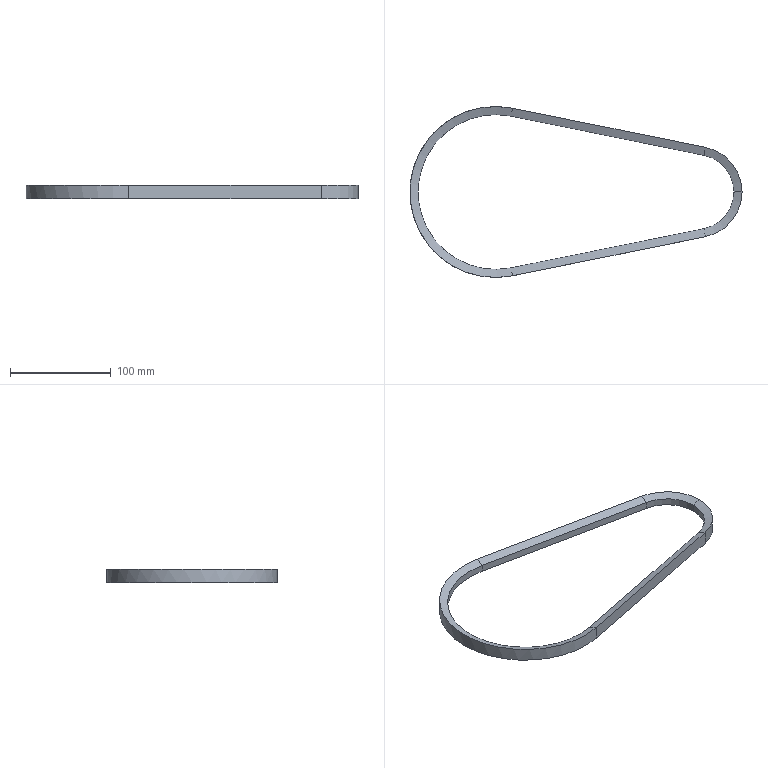Part | SolidWorks | features Sweep 1 | 1 solid | 20 faces | box 329.455 x 169.695 x 13 mm | volume 63968 mm3 | plane 8 | cone 6 | cylinder 6 | commonest cylinder face diameters 74.495 x2 90.495 x2 153.695 x1 169.695 x1
STEP:
#1=CARTESIAN_POINT('',(-184.095,75.316,-3.588));
#2=VERTEX_POINT('',#1);
#3=CARTESIAN_POINT('',(-276.207,0.,-3.588));
#4=VERTEX_POINT('',#3);
#5=CARTESIAN_POINT('',(-199.36,0.,-3.588));
#6=DIRECTION('',(0.,0.,1.));
#7=DIRECTION('',(1.,0.,0.));
#8=AXIS2_PLACEMENT_3D('',#5,#6,#7);
#9=CIRCLE('',#8,76.847);
#10=EDGE_CURVE('',#2,#4,#9,.T.);
#11=ORIENTED_EDGE('',*,*,#10,.T.);
#12=CARTESIAN_POINT('',(-284.207,0.,-6.5));
#13=VERTEX_POINT('',#12);
#14=CARTESIAN_POINT('',(-276.207,0.,-3.588));
#15=DIRECTION('',(-0.9397,0.,-0.342));
#16=VECTOR('',#15,1000.);
#17=LINE('',#14,#16);
#18=EDGE_CURVE('',#4,#13,#17,.T.);
#19=ORIENTED_EDGE('',*,*,#18,.T.);
#20=CARTESIAN_POINT('',(-182.506,83.157,-6.5));
#21=VERTEX_POINT('',#20);
#22=CARTESIAN_POINT('',(-199.36,0.,-6.5));
#23=DIRECTION('',(0.,0.,1.));
#24=DIRECTION('',(1.,0.,0.));
#25=AXIS2_PLACEMENT_3D('',#22,#23,#24);
#26=CIRCLE('',#25,84.847);
#27=EDGE_CURVE('',#21,#13,#26,.T.);
#28=ORIENTED_EDGE('',*,*,#27,.F.);
#29=CARTESIAN_POINT('',(-183.052,80.464,-5.5));
#30=DIRECTION('',(0.1867,0.921,-0.342));
#31=VECTOR('',#30,1000.);
#32=LINE('',#29,#31);
#33=EDGE_CURVE('',#2,#21,#32,.T.);
#34=ORIENTED_EDGE('',*,*,#33,.F.);
#35=EDGE_LOOP('',(#11,#19,#28,#34));
#36=FACE_OUTER_BOUND('',#35,.T.);
#37=CARTESIAN_POINT('',(-199.36,0.,-3.588));
#38=DIRECTION('',(0.,0.,-1.));
#39=DIRECTION('',(-1.,0.,0.));
#40=AXIS2_PLACEMENT_3D('',#37,#38,#39);
#41=CONICAL_SURFACE('',#40,76.847,1.222);
#42=ADVANCED_FACE('',(#36),#41,.F.);
#43=CARTESIAN_POINT('',(8.988,-44.346,-6.5));
#44=VERTEX_POINT('',#43);
#45=CARTESIAN_POINT('',(45.247,0.,-6.5));
#46=VERTEX_POINT('',#45);
#47=CARTESIAN_POINT('',(0.,0.,-6.5));
#48=DIRECTION('',(0.,0.,1.));
#49=DIRECTION('',(1.,0.,0.));
#50=AXIS2_PLACEMENT_3D('',#47,#48,#49);
#51=CIRCLE('',#50,45.247);
#52=EDGE_CURVE('',#44,#46,#51,.T.);
#53=ORIENTED_EDGE('',*,*,#52,.T.);
#54=CARTESIAN_POINT('',(45.247,0.,6.5));
#55=VERTEX_POINT('',#54);
#56=CARTESIAN_POINT('',(45.247,0.,0.));
#57=DIRECTION('',(0.,0.,1.));
#58=VECTOR('',#57,1000.);
#59=LINE('',#56,#58);
#60=EDGE_CURVE('',#46,#55,#59,.T.);
#61=ORIENTED_EDGE('',*,*,#60,.T.);
#62=CARTESIAN_POINT('',(8.988,-44.346,6.5));
#63=VERTEX_POINT('',#62);
#64=CARTESIAN_POINT('',(0.,0.,6.5));
#65=DIRECTION('',(0.,0.,1.));
#66=DIRECTION('',(1.,0.,0.));
#67=AXIS2_PLACEMENT_3D('',#64,#65,#66);
#68=CIRCLE('',#67,45.247);
#69=EDGE_CURVE('',#63,#55,#68,.T.);
#70=ORIENTED_EDGE('',*,*,#69,.F.);
#71=CARTESIAN_POINT('',(8.988,-44.346,-6.5));
#72=DIRECTION('',(0.,0.,1.));
#73=VECTOR('',#72,1000.);
#74=LINE('',#71,#73);
#75=EDGE_CURVE('',#44,#63,#74,.T.);
#76=ORIENTED_EDGE('',*,*,#75,.F.);
#77=EDGE_LOOP('',(#53,#61,#70,#76));
#78=FACE_OUTER_BOUND('',#77,.T.);
#79=CARTESIAN_POINT('',(0.,0.,0.));
#80=DIRECTION('',(0.,0.,1.));
#81=DIRECTION('',(1.,0.,0.));
#82=AXIS2_PLACEMENT_3D('',#79,#80,#81);
#83=CYLINDRICAL_SURFACE('',#82,45.247);
#84=ADVANCED_FACE('',(#78),#83,.T.);
#85=CARTESIAN_POINT('',(37.247,0.,3.588));
#86=VERTEX_POINT('',#85);
#87=CARTESIAN_POINT('',(7.399,36.505,3.588));
#88=VERTEX_POINT('',#87);
#89=CARTESIAN_POINT('',(0.,0.,3.588));
#90=DIRECTION('',(0.,0.,1.));
#91=DIRECTION('',(1.,0.,0.));
#92=AXIS2_PLACEMENT_3D('',#89,#90,#91);
#93=CIRCLE('',#92,37.247);
#94=EDGE_CURVE('',#86,#88,#93,.T.);
#95=ORIENTED_EDGE('',*,*,#94,.F.);
#96=CARTESIAN_POINT('',(45.247,0.,6.5));
#97=DIRECTION('',(0.9397,0.,0.342));
#98=VECTOR('',#97,1000.);
#99=LINE('',#96,#98);
#100=EDGE_CURVE('',#86,#55,#99,.T.);
#101=ORIENTED_EDGE('',*,*,#100,.T.);
#102=CARTESIAN_POINT('',(8.988,44.346,6.5));
#103=VERTEX_POINT('',#102);
#104=CARTESIAN_POINT('',(0.,0.,6.5));
#105=DIRECTION('',(0.,0.,1.));
#106=DIRECTION('',(1.,0.,0.));
#107=AXIS2_PLACEMENT_3D('',#104,#105,#106);
#108=CIRCLE('',#107,45.247);
#109=EDGE_CURVE('',#55,#103,#108,.T.);
#110=ORIENTED_EDGE('',*,*,#109,.T.);
#111=CARTESIAN_POINT('',(8.442,41.653,5.5));
#112=VERTEX_POINT('',#111);
#113=CARTESIAN_POINT('',(8.988,44.346,6.5));
#114=CARTESIAN_POINT('',(8.806,43.448,6.167));
#115=CARTESIAN_POINT('',(8.624,42.551,5.833));
#116=CARTESIAN_POINT('',(8.442,41.653,5.5));
#117=B_SPLINE_CURVE_WITH_KNOTS('',3,(#113,#114,#115,#116),.UNSPECIFIED.,.F.,.F.,(4,4),(0.,1.),.UNSPECIFIED.);
#118=EDGE_CURVE('',#103,#112,#117,.T.);
#119=ORIENTED_EDGE('',*,*,#118,.T.);
#120=CARTESIAN_POINT('',(8.442,41.653,5.5));
#121=CARTESIAN_POINT('',(8.094,39.937,4.863));
#122=CARTESIAN_POINT('',(7.746,38.221,4.225));
#123=CARTESIAN_POINT('',(7.399,36.505,3.588));
#124=B_SPLINE_CURVE_WITH_KNOTS('',3,(#120,#121,#122,#123),.UNSPECIFIED.,.F.,.F.,(4,4),(0.,1.),.UNSPECIFIED.);
#125=EDGE_CURVE('',#112,#88,#124,.T.);
#126=ORIENTED_EDGE('',*,*,#125,.T.);
#127=EDGE_LOOP('',(#95,#101,#110,#119,#126));
#128=FACE_OUTER_BOUND('',#127,.T.);
#129=CARTESIAN_POINT('',(0.,0.,6.5));
#130=DIRECTION('',(0.,0.,1.));
#131=DIRECTION('',(1.,0.,0.));
#132=AXIS2_PLACEMENT_3D('',#129,#130,#131);
#133=CONICAL_SURFACE('',#132,45.247,1.222);
#134=ADVANCED_FACE('',(#128),#133,.F.);
#135=CARTESIAN_POINT('',(37.247,0.,-3.588));
#136=VERTEX_POINT('',#135);
#137=CARTESIAN_POINT('',(7.399,36.505,-3.588));
#138=VERTEX_POINT('',#137);
#139=CARTESIAN_POINT('',(0.,0.,-3.588));
#140=DIRECTION('',(0.,0.,1.));
#141=DIRECTION('',(1.,0.,0.));
#142=AXIS2_PLACEMENT_3D('',#139,#140,#141);
#143=CIRCLE('',#142,37.247);
#144=EDGE_CURVE('',#136,#138,#143,.T.);
#145=ORIENTED_EDGE('',*,*,#144,.F.);
#146=CARTESIAN_POINT('',(37.247,0.,0.));
#147=DIRECTION('',(0.,0.,1.));
#148=VECTOR('',#147,1000.);
#149=LINE('',#146,#148);
#150=EDGE_CURVE('',#136,#86,#149,.T.);
#151=ORIENTED_EDGE('',*,*,#150,.T.);
#152=ORIENTED_EDGE('',*,*,#94,.T.);
#153=CARTESIAN_POINT('',(7.399,36.505,3.588));
#154=CARTESIAN_POINT('',(7.399,36.505,1.196));
#155=CARTESIAN_POINT('',(7.399,36.505,-1.196));
#156=CARTESIAN_POINT('',(7.399,36.505,-3.588));
#157=B_SPLINE_CURVE_WITH_KNOTS('',3,(#153,#154,#155,#156),.UNSPECIFIED.,.F.,.F.,(4,4),(0.,1.),.UNSPECIFIED.);
#158=EDGE_CURVE('',#88,#138,#157,.T.);
#159=ORIENTED_EDGE('',*,*,#158,.T.);
#160=EDGE_LOOP('',(#145,#151,#152,#159));
#161=FACE_OUTER_BOUND('',#160,.T.);
#162=CARTESIAN_POINT('',(0.,0.,0.));
#163=DIRECTION('',(0.,0.,1.));
#164=DIRECTION('',(1.,0.,0.));
#165=AXIS2_PLACEMENT_3D('',#162,#163,#164);
#166=CYLINDRICAL_SURFACE('',#165,37.247);
#167=ADVANCED_FACE('',(#161),#166,.F.);
#168=ORIENTED_EDGE('',*,*,#150,.F.);
#169=CARTESIAN_POINT('',(7.399,-36.505,-3.588));
#170=VERTEX_POINT('',#169);
#171=CARTESIAN_POINT('',(0.,0.,-3.588));
#172=DIRECTION('',(0.,0.,1.));
#173=DIRECTION('',(1.,0.,0.));
#174=AXIS2_PLACEMENT_3D('',#171,#172,#173);
#175=CIRCLE('',#174,37.247);
#176=EDGE_CURVE('',#170,#136,#175,.T.);
#177=ORIENTED_EDGE('',*,*,#176,.F.);
#178=CARTESIAN_POINT('',(7.399,-36.505,3.588));
#179=VERTEX_POINT('',#178);
#180=CARTESIAN_POINT('',(7.399,-36.505,3.588));
#181=DIRECTION('',(0.,0.,-1.));
#182=VECTOR('',#181,1000.);
#183=LINE('',#180,#182);
#184=EDGE_CURVE('',#179,#170,#183,.T.);
#185=ORIENTED_EDGE('',*,*,#184,.F.);
#186=CARTESIAN_POINT('',(0.,0.,3.588));
#187=DIRECTION('',(0.,0.,1.));
#188=DIRECTION('',(1.,0.,0.));
#189=AXIS2_PLACEMENT_3D('',#186,#187,#188);
#190=CIRCLE('',#189,37.247);
#191=EDGE_CURVE('',#179,#86,#190,.T.);
#192=ORIENTED_EDGE('',*,*,#191,.T.);
#193=EDGE_LOOP('',(#168,#177,#185,#192));
#194=FACE_OUTER_BOUND('',#193,.T.);
#195=CARTESIAN_POINT('',(0.,0.,0.));
#196=DIRECTION('',(0.,0.,1.));
#197=DIRECTION('',(1.,0.,0.));
#198=AXIS2_PLACEMENT_3D('',#195,#196,#197);
#199=CYLINDRICAL_SURFACE('',#198,37.247);
#200=ADVANCED_FACE('',(#194),#199,.F.);
#201=ORIENTED_EDGE('',*,*,#100,.F.);
#202=ORIENTED_EDGE('',*,*,#191,.F.);
#203=CARTESIAN_POINT('',(8.442,-41.653,5.5));
#204=DIRECTION('',(-0.1867,0.921,-0.342));
#205=VECTOR('',#204,1000.);
#206=LINE('',#203,#205);
#207=EDGE_CURVE('',#63,#179,#206,.T.);
#208=ORIENTED_EDGE('',*,*,#207,.F.);
#209=ORIENTED_EDGE('',*,*,#69,.T.);
#210=EDGE_LOOP('',(#201,#202,#208,#209));
#211=FACE_OUTER_BOUND('',#210,.T.);
#212=CARTESIAN_POINT('',(0.,0.,6.5));
#213=DIRECTION('',(0.,0.,1.));
#214=DIRECTION('',(1.,0.,0.));
#215=AXIS2_PLACEMENT_3D('',#212,#213,#214);
#216=CONICAL_SURFACE('',#215,45.247,1.222);
#217=ADVANCED_FACE('',(#211),#216,.F.);
#218=ORIENTED_EDGE('',*,*,#60,.F.);
#219=CARTESIAN_POINT('',(8.988,44.346,-6.5));
#220=VERTEX_POINT('',#219);
#221=CARTESIAN_POINT('',(0.,0.,-6.5));
#222=DIRECTION('',(0.,0.,1.));
#223=DIRECTION('',(1.,0.,0.));
#224=AXIS2_PLACEMENT_3D('',#221,#222,#223);
#225=CIRCLE('',#224,45.247);
#226=EDGE_CURVE('',#46,#220,#225,.T.);
#227=ORIENTED_EDGE('',*,*,#226,.T.);
#228=CARTESIAN_POINT('',(8.988,44.346,-6.5));
#229=CARTESIAN_POINT('',(8.988,44.346,-2.167));
#230=CARTESIAN_POINT('',(8.988,44.346,2.167));
#231=CARTESIAN_POINT('',(8.988,44.346,6.5));
#232=B_SPLINE_CURVE_WITH_KNOTS('',3,(#228,#229,#230,#231),.UNSPECIFIED.,.F.,.F.,(4,4),(0.,1.),.UNSPECIFIED.);
#233=EDGE_CURVE('',#220,#103,#232,.T.);
#234=ORIENTED_EDGE('',*,*,#233,.T.);
#235=ORIENTED_EDGE('',*,*,#109,.F.);
#236=EDGE_LOOP('',(#218,#227,#234,#235));
#237=FACE_OUTER_BOUND('',#236,.T.);
#238=CARTESIAN_POINT('',(0.,0.,0.));
#239=DIRECTION('',(0.,0.,1.));
#240=DIRECTION('',(1.,0.,0.));
#241=AXIS2_PLACEMENT_3D('',#238,#239,#240);
#242=CYLINDRICAL_SURFACE('',#241,45.247);
#243=ADVANCED_FACE('',(#237),#242,.T.);
#244=CARTESIAN_POINT('',(8.442,-41.653,-5.5));
#245=DIRECTION('',(0.1867,-0.921,-0.342));
#246=VECTOR('',#245,1000.);
#247=LINE('',#244,#246);
#248=EDGE_CURVE('',#170,#44,#247,.T.);
#249=ORIENTED_EDGE('',*,*,#248,.F.);
#250=ORIENTED_EDGE('',*,*,#176,.T.);
#251=ORIENTED_EDGE('',*,*,#144,.T.);
#252=CARTESIAN_POINT('',(8.442,41.653,-5.5));
#253=VERTEX_POINT('',#252);
#254=CARTESIAN_POINT('',(7.399,36.505,-3.588));
#255=CARTESIAN_POINT('',(7.746,38.221,-4.225));
#256=CARTESIAN_POINT('',(8.094,39.937,-4.863));
#257=CARTESIAN_POINT('',(8.442,41.653,-5.5));
#258=B_SPLINE_CURVE_WITH_KNOTS('',3,(#254,#255,#256,#257),.UNSPECIFIED.,.F.,.F.,(4,4),(0.,1.),.UNSPECIFIED.);
#259=EDGE_CURVE('',#138,#253,#258,.T.);
#260=ORIENTED_EDGE('',*,*,#259,.T.);
#261=CARTESIAN_POINT('',(8.442,41.653,-5.5));
#262=CARTESIAN_POINT('',(8.624,42.551,-5.833));
#263=CARTESIAN_POINT('',(8.806,43.448,-6.167));
#264=CARTESIAN_POINT('',(8.988,44.346,-6.5));
#265=B_SPLINE_CURVE_WITH_KNOTS('',3,(#261,#262,#263,#264),.UNSPECIFIED.,.F.,.F.,(4,4),(0.,1.),.UNSPECIFIED.);
#266=EDGE_CURVE('',#253,#220,#265,.T.);
#267=ORIENTED_EDGE('',*,*,#266,.T.);
#268=ORIENTED_EDGE('',*,*,#226,.F.);
#269=ORIENTED_EDGE('',*,*,#52,.F.);
#270=EDGE_LOOP('',(#249,#250,#251,#260,#267,#268,#269));
#271=FACE_OUTER_BOUND('',#270,.T.);
#272=CARTESIAN_POINT('',(0.,0.,-3.588));
#273=DIRECTION('',(0.,0.,-1.));
#274=DIRECTION('',(-1.,0.,0.));
#275=AXIS2_PLACEMENT_3D('',#272,#273,#274);
#276=CONICAL_SURFACE('',#275,37.247,1.222);
#277=ADVANCED_FACE('',(#271),#276,.F.);
#278=CARTESIAN_POINT('',(-184.095,-75.316,3.588));
#279=VERTEX_POINT('',#278);
#280=CARTESIAN_POINT('',(-184.095,-75.316,-3.588));
#281=VERTEX_POINT('',#280);
#282=CARTESIAN_POINT('',(-184.095,-75.316,3.588));
#283=DIRECTION('',(0.,0.,-1.));
#284=VECTOR('',#283,1000.);
#285=LINE('',#282,#284);
#286=EDGE_CURVE('',#279,#281,#285,.T.);
#287=ORIENTED_EDGE('',*,*,#286,.F.);
#288=CARTESIAN_POINT('',(-184.095,-75.316,3.588));
#289=DIRECTION('',(0.9801,0.1986,0.));
#290=VECTOR('',#289,1000.);
#291=LINE('',#288,#290);
#292=EDGE_CURVE('',#279,#179,#291,.T.);
#293=ORIENTED_EDGE('',*,*,#292,.T.);
#294=ORIENTED_EDGE('',*,*,#184,.T.);
#295=CARTESIAN_POINT('',(-184.095,-75.316,-3.588));
#296=DIRECTION('',(0.9801,0.1986,0.));
#297=VECTOR('',#296,1000.);
#298=LINE('',#295,#297);
#299=EDGE_CURVE('',#281,#170,#298,.T.);
#300=ORIENTED_EDGE('',*,*,#299,.F.);
#301=EDGE_LOOP('',(#287,#293,#294,#300));
#302=FACE_OUTER_BOUND('',#301,.T.);
#303=CARTESIAN_POINT('',(-184.095,-75.316,3.588));
#304=DIRECTION('',(0.1986,-0.9801,0.));
#305=DIRECTION('',(0.9801,0.1986,0.));
#306=AXIS2_PLACEMENT_3D('',#303,#304,#305);
#307=PLANE('',#306);
#308=ADVANCED_FACE('',(#302),#307,.F.);
#309=CARTESIAN_POINT('',(-182.506,-83.157,6.5));
#310=VERTEX_POINT('',#309);
#311=CARTESIAN_POINT('',(-183.052,-80.464,5.5));
#312=DIRECTION('',(-0.1867,0.921,-0.342));
#313=VECTOR('',#312,1000.);
#314=LINE('',#311,#313);
#315=EDGE_CURVE('',#310,#279,#314,.T.);
#316=ORIENTED_EDGE('',*,*,#315,.F.);
#317=CARTESIAN_POINT('',(-182.506,-83.157,6.5));
#318=DIRECTION('',(0.9801,0.1986,0.));
#319=VECTOR('',#318,1000.);
#320=LINE('',#317,#319);
#321=EDGE_CURVE('',#310,#63,#320,.T.);
#322=ORIENTED_EDGE('',*,*,#321,.T.);
#323=ORIENTED_EDGE('',*,*,#207,.T.);
#324=ORIENTED_EDGE('',*,*,#292,.F.);
#325=EDGE_LOOP('',(#316,#322,#323,#324));
#326=FACE_OUTER_BOUND('',#325,.T.);
#327=CARTESIAN_POINT('',(-183.052,-80.464,5.5));
#328=DIRECTION('',(0.06794,-0.3352,-0.9397));
#329=DIRECTION('',(0.,0.9419,-0.336));
#330=AXIS2_PLACEMENT_3D('',#327,#328,#329);
#331=PLANE('',#330);
#332=ADVANCED_FACE('',(#326),#331,.F.);
#333=CARTESIAN_POINT('',(-182.506,-83.157,-6.5));
#334=VERTEX_POINT('',#333);
#335=CARTESIAN_POINT('',(-182.506,-83.157,-6.5));
#336=DIRECTION('',(0.,0.,1.));
#337=VECTOR('',#336,1000.);
#338=LINE('',#335,#337);
#339=EDGE_CURVE('',#334,#310,#338,.T.);
#340=ORIENTED_EDGE('',*,*,#339,.F.);
#341=CARTESIAN_POINT('',(-182.506,-83.157,-6.5));
#342=DIRECTION('',(0.9801,0.1986,0.));
#343=VECTOR('',#342,1000.);
#344=LINE('',#341,#343);
#345=EDGE_CURVE('',#334,#44,#344,.T.);
#346=ORIENTED_EDGE('',*,*,#345,.T.);
#347=ORIENTED_EDGE('',*,*,#75,.T.);
#348=ORIENTED_EDGE('',*,*,#321,.F.);
#349=EDGE_LOOP('',(#340,#346,#347,#348));
#350=FACE_OUTER_BOUND('',#349,.T.);
#351=CARTESIAN_POINT('',(-182.506,-83.157,-6.5));
#352=DIRECTION('',(-0.1986,0.9801,0.));
#353=DIRECTION('',(-0.9801,-0.1986,0.));
#354=AXIS2_PLACEMENT_3D('',#351,#352,#353);
#355=PLANE('',#354);
#356=ADVANCED_FACE('',(#350),#355,.F.);
#357=CARTESIAN_POINT('',(-183.052,-80.464,-5.5));
#358=DIRECTION('',(0.1867,-0.921,-0.342));
#359=VECTOR('',#358,1000.);
#360=LINE('',#357,#359);
#361=EDGE_CURVE('',#281,#334,#360,.T.);
#362=ORIENTED_EDGE('',*,*,#361,.F.);
#363=ORIENTED_EDGE('',*,*,#299,.T.);
#364=ORIENTED_EDGE('',*,*,#248,.T.);
#365=ORIENTED_EDGE('',*,*,#345,.F.);
#366=EDGE_LOOP('',(#362,#363,#364,#365));
#367=FACE_OUTER_BOUND('',#366,.T.);
#368=CARTESIAN_POINT('',(-183.052,-80.464,-5.5));
#369=DIRECTION('',(0.06794,-0.3352,0.9397));
#370=DIRECTION('',(0.,-0.9419,-0.336));
#371=AXIS2_PLACEMENT_3D('',#368,#369,#370);
#372=PLANE('',#371);
#373=ADVANCED_FACE('',(#367),#372,.F.);
#374=CARTESIAN_POINT('',(-184.095,75.316,3.588));
#375=VERTEX_POINT('',#374);
#376=CARTESIAN_POINT('',(-184.095,75.316,3.588));
#377=DIRECTION('',(0.,0.,-1.));
#378=VECTOR('',#377,1000.);
#379=LINE('',#376,#378);
#380=EDGE_CURVE('',#375,#2,#379,.T.);
#381=ORIENTED_EDGE('',*,*,#380,.F.);
#382=CARTESIAN_POINT('',(-199.36,0.,3.588));
#383=DIRECTION('',(0.,0.,1.));
#384=DIRECTION('',(1.,0.,0.));
#385=AXIS2_PLACEMENT_3D('',#382,#383,#384);
#386=CIRCLE('',#385,76.847);
#387=EDGE_CURVE('',#375,#279,#386,.T.);
#388=ORIENTED_EDGE('',*,*,#387,.T.);
#389=ORIENTED_EDGE('',*,*,#286,.T.);
#390=CARTESIAN_POINT('',(-199.36,0.,-3.588));
#391=DIRECTION('',(0.,0.,1.));
#392=DIRECTION('',(1.,0.,0.));
#393=AXIS2_PLACEMENT_3D('',#390,#391,#392);
#394=CIRCLE('',#393,76.847);
#395=EDGE_CURVE('',#4,#281,#394,.T.);
#396=ORIENTED_EDGE('',*,*,#395,.F.);
#397=ORIENTED_EDGE('',*,*,#10,.F.);
#398=EDGE_LOOP('',(#381,#388,#389,#396,#397));
#399=FACE_OUTER_BOUND('',#398,.T.);
#400=CARTESIAN_POINT('',(-199.36,0.,0.));
#401=DIRECTION('',(0.,0.,1.));
#402=DIRECTION('',(1.,0.,0.));
#403=AXIS2_PLACEMENT_3D('',#400,#401,#402);
#404=CYLINDRICAL_SURFACE('',#403,76.847);
#405=ADVANCED_FACE('',(#399),#404,.F.);
#406=CARTESIAN_POINT('',(-182.506,83.157,6.5));
#407=VERTEX_POINT('',#406);
#408=CARTESIAN_POINT('',(-183.052,80.464,5.5));
#409=DIRECTION('',(-0.1867,-0.921,-0.342));
#410=VECTOR('',#409,1000.);
#411=LINE('',#408,#410);
#412=EDGE_CURVE('',#407,#375,#411,.T.);
#413=ORIENTED_EDGE('',*,*,#412,.F.);
#414=CARTESIAN_POINT('',(-199.36,0.,6.5));
#415=DIRECTION('',(0.,0.,1.));
#416=DIRECTION('',(1.,0.,0.));
#417=AXIS2_PLACEMENT_3D('',#414,#415,#416);
#418=CIRCLE('',#417,84.847);
#419=EDGE_CURVE('',#407,#310,#418,.T.);
#420=ORIENTED_EDGE('',*,*,#419,.T.);
#421=ORIENTED_EDGE('',*,*,#315,.T.);
#422=ORIENTED_EDGE('',*,*,#387,.F.);
#423=EDGE_LOOP('',(#413,#420,#421,#422));
#424=FACE_OUTER_BOUND('',#423,.T.);
#425=CARTESIAN_POINT('',(-199.36,0.,6.5));
#426=DIRECTION('',(0.,0.,1.));
#427=DIRECTION('',(1.,0.,0.));
#428=AXIS2_PLACEMENT_3D('',#425,#426,#427);
#429=CONICAL_SURFACE('',#428,84.847,1.222);
#430=ADVANCED_FACE('',(#424),#429,.F.);
#431=CARTESIAN_POINT('',(-182.506,83.157,-6.5));
#432=DIRECTION('',(0.,0.,1.));
#433=VECTOR('',#432,1000.);
#434=LINE('',#431,#433);
#435=EDGE_CURVE('',#21,#407,#434,.T.);
#436=ORIENTED_EDGE('',*,*,#435,.F.);
#437=ORIENTED_EDGE('',*,*,#27,.T.);
#438=CARTESIAN_POINT('',(-199.36,0.,-6.5));
#439=DIRECTION('',(0.,0.,1.));
#440=DIRECTION('',(1.,0.,0.));
#441=AXIS2_PLACEMENT_3D('',#438,#439,#440);
#442=CIRCLE('',#441,84.847);
#443=EDGE_CURVE('',#13,#334,#442,.T.);
#444=ORIENTED_EDGE('',*,*,#443,.T.);
#445=ORIENTED_EDGE('',*,*,#339,.T.);
#446=ORIENTED_EDGE('',*,*,#419,.F.);
#447=EDGE_LOOP('',(#436,#437,#444,#445,#446));
#448=FACE_OUTER_BOUND('',#447,.T.);
#449=CARTESIAN_POINT('',(-199.36,0.,0.));
#450=DIRECTION('',(0.,0.,1.));
#451=DIRECTION('',(1.,0.,0.));
#452=AXIS2_PLACEMENT_3D('',#449,#450,#451);
#453=CYLINDRICAL_SURFACE('',#452,84.847);
#454=ADVANCED_FACE('',(#448),#453,.T.);
#455=ORIENTED_EDGE('',*,*,#18,.F.);
#456=ORIENTED_EDGE('',*,*,#395,.T.);
#457=ORIENTED_EDGE('',*,*,#361,.T.);
#458=ORIENTED_EDGE('',*,*,#443,.F.);
#459=EDGE_LOOP('',(#455,#456,#457,#458));
#460=FACE_OUTER_BOUND('',#459,.T.);
#461=CARTESIAN_POINT('',(-199.36,0.,-3.588));
#462=DIRECTION('',(0.,0.,-1.));
#463=DIRECTION('',(-1.,0.,0.));
#464=AXIS2_PLACEMENT_3D('',#461,#462,#463);
#465=CONICAL_SURFACE('',#464,76.847,1.222);
#466=ADVANCED_FACE('',(#460),#465,.F.);
#467=ORIENTED_EDGE('',*,*,#158,.F.);
#468=CARTESIAN_POINT('',(-184.095,75.316,3.588));
#469=DIRECTION('',(0.9801,-0.1986,0.));
#470=VECTOR('',#469,1000.);
#471=LINE('',#468,#470);
#472=EDGE_CURVE('',#375,#88,#471,.T.);
#473=ORIENTED_EDGE('',*,*,#472,.F.);
#474=ORIENTED_EDGE('',*,*,#380,.T.);
#475=CARTESIAN_POINT('',(-184.095,75.316,-3.588));
#476=DIRECTION('',(0.9801,-0.1986,0.));
#477=VECTOR('',#476,1000.);
#478=LINE('',#475,#477);
#479=EDGE_CURVE('',#2,#138,#478,.T.);
#480=ORIENTED_EDGE('',*,*,#479,.T.);
#481=EDGE_LOOP('',(#467,#473,#474,#480));
#482=FACE_OUTER_BOUND('',#481,.T.);
#483=CARTESIAN_POINT('',(-184.095,75.316,3.588));
#484=DIRECTION('',(-0.1986,-0.9801,0.));
#485=DIRECTION('',(0.9801,-0.1986,0.));
#486=AXIS2_PLACEMENT_3D('',#483,#484,#485);
#487=PLANE('',#486);
#488=ADVANCED_FACE('',(#482),#487,.T.);
#489=ORIENTED_EDGE('',*,*,#125,.F.);
#490=ORIENTED_EDGE('',*,*,#118,.F.);
#491=CARTESIAN_POINT('',(-182.506,83.157,6.5));
#492=DIRECTION('',(0.9801,-0.1986,0.));
#493=VECTOR('',#492,1000.);
#494=LINE('',#491,#493);
#495=EDGE_CURVE('',#407,#103,#494,.T.);
#496=ORIENTED_EDGE('',*,*,#495,.F.);
#497=ORIENTED_EDGE('',*,*,#412,.T.);
#498=ORIENTED_EDGE('',*,*,#472,.T.);
#499=EDGE_LOOP('',(#489,#490,#496,#497,#498));
#500=FACE_OUTER_BOUND('',#499,.T.);
#501=CARTESIAN_POINT('',(-183.052,80.464,5.5));
#502=DIRECTION('',(-0.06794,-0.3352,0.9397));
#503=DIRECTION('',(0.,-0.9419,-0.336));
#504=AXIS2_PLACEMENT_3D('',#501,#502,#503);
#505=PLANE('',#504);
#506=ADVANCED_FACE('',(#500),#505,.T.);
#507=ORIENTED_EDGE('',*,*,#233,.F.);
#508=CARTESIAN_POINT('',(-182.506,83.157,-6.5));
#509=DIRECTION('',(0.9801,-0.1986,0.));
#510=VECTOR('',#509,1000.);
#511=LINE('',#508,#510);
#512=EDGE_CURVE('',#21,#220,#511,.T.);
#513=ORIENTED_EDGE('',*,*,#512,.F.);
#514=ORIENTED_EDGE('',*,*,#435,.T.);
#515=ORIENTED_EDGE('',*,*,#495,.T.);
#516=EDGE_LOOP('',(#507,#513,#514,#515));
#517=FACE_OUTER_BOUND('',#516,.T.);
#518=CARTESIAN_POINT('',(-182.506,83.157,-6.5));
#519=DIRECTION('',(0.1986,0.9801,0.));
#520=DIRECTION('',(-0.9801,0.1986,0.));
#521=AXIS2_PLACEMENT_3D('',#518,#519,#520);
#522=PLANE('',#521);
#523=ADVANCED_FACE('',(#517),#522,.T.);
#524=ORIENTED_EDGE('',*,*,#266,.F.);
#525=ORIENTED_EDGE('',*,*,#259,.F.);
#526=ORIENTED_EDGE('',*,*,#479,.F.);
#527=ORIENTED_EDGE('',*,*,#33,.T.);
#528=ORIENTED_EDGE('',*,*,#512,.T.);
#529=EDGE_LOOP('',(#524,#525,#526,#527,#528));
#530=FACE_OUTER_BOUND('',#529,.T.);
#531=CARTESIAN_POINT('',(-183.052,80.464,-5.5));
#532=DIRECTION('',(-0.06794,-0.3352,-0.9397));
#533=DIRECTION('',(0.,0.9419,-0.336));
#534=AXIS2_PLACEMENT_3D('',#531,#532,#533);
#535=PLANE('',#534);
#536=ADVANCED_FACE('',(#530),#535,.T.);
#537=CLOSED_SHELL('',(#42,#84,#134,#167,#200,#217,#243,#277,#308,#332,#356,#373,#405,#430,#454,#466,#488,#506,#523,#536));
#538=MANIFOLD_SOLID_BREP('',#537);
#539=CARTESIAN_POINT('',(0.,0.,0.));
#540=DIRECTION('',(0.,0.,1.));
#541=DIRECTION('',(1.,0.,0.));
#542=AXIS2_PLACEMENT_3D('',#539,#540,#541);
#543=(LENGTH_UNIT()NAMED_UNIT(*)SI_UNIT(.MILLI.,.METRE.));
#544=UNCERTAINTY_MEASURE_WITH_UNIT(LENGTH_MEASURE(0.00001),#543,'','');
#545=(NAMED_UNIT(*)PLANE_ANGLE_UNIT()SI_UNIT($,.RADIAN.));
#546=(NAMED_UNIT(*)SI_UNIT($,.STERADIAN.)SOLID_ANGLE_UNIT());
#547=(GEOMETRIC_REPRESENTATION_CONTEXT(3)GLOBAL_UNCERTAINTY_ASSIGNED_CONTEXT((#544))GLOBAL_UNIT_ASSIGNED_CONTEXT((#543,#545,#546))REPRESENTATION_CONTEXT('',''));
#548=ADVANCED_BREP_SHAPE_REPRESENTATION('',(#538,#542),#547);